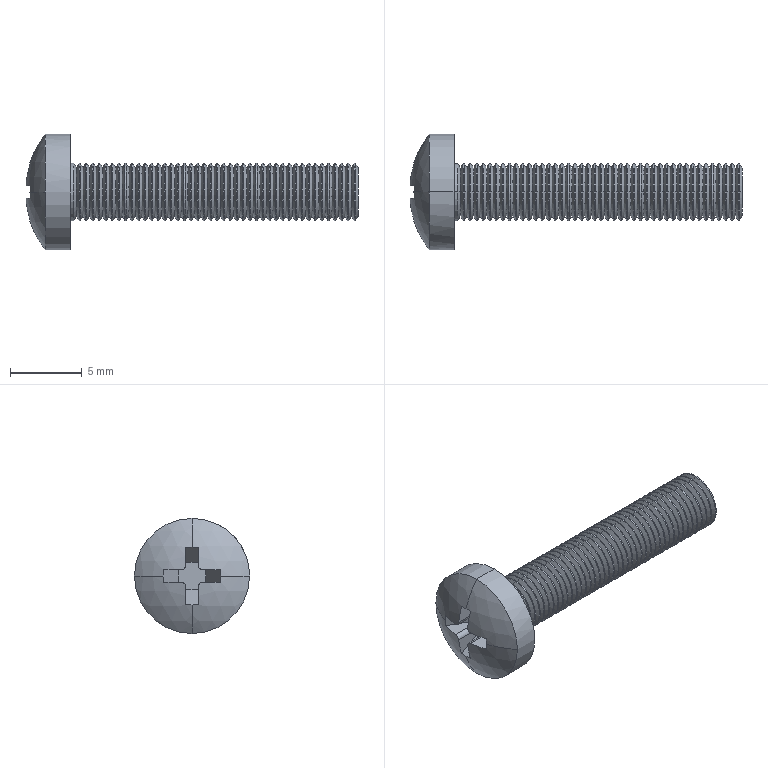Part | STEP file | 46A-01001LS15_Default<As Machined> | 1 solid | 287 faces | box 23.057 x 8 x 8 mm | volume 332.138 mm3 | cone 174 | cylinder 94 | plane 15 | sphere 4 | commonest cylinder face diameters 4 x88 0.6 x4 8 x2